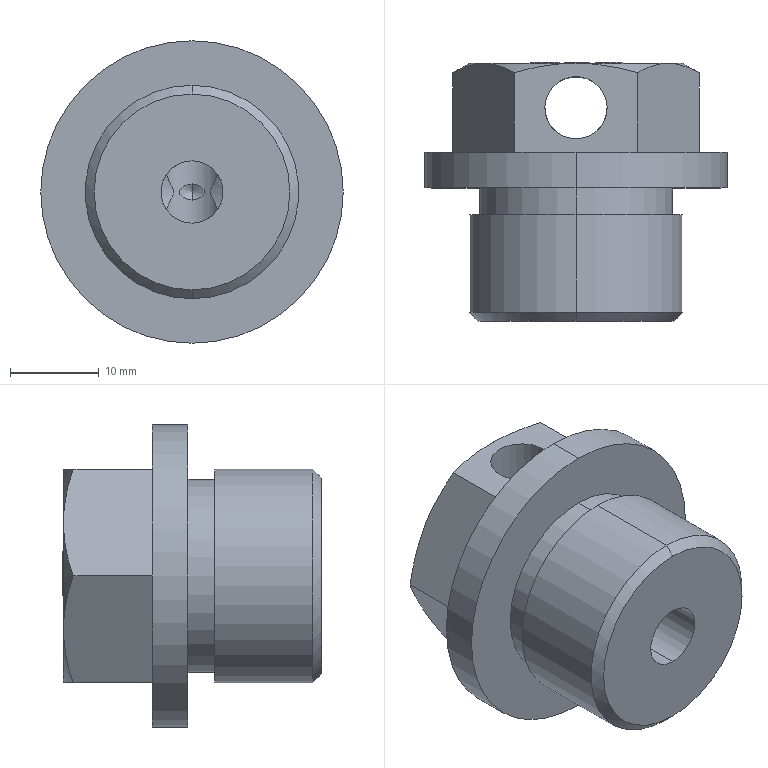Part | SolidWorks | features ICE 2, RevCut 2, Chamfer 1, Extrusion 1, Revolution 1 | 1 solid | 344 faces | box 34 x 29.1 x 34 mm | volume 13367 mm3 | plane 221 | spline 98 | cylinder 13 | cone 12 | commonest cylinder face diameters 7 x7 21.7 x2 24 x2 34 x2